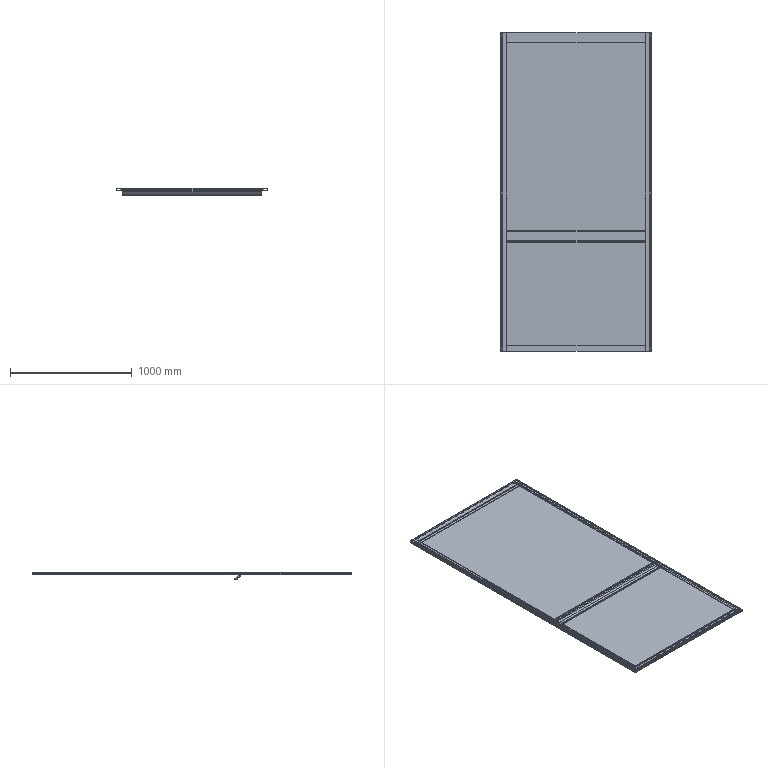Part | 13 solids | 642 faces | box 1240 x 2616 x 63.186 mm | volume 31579551 mm3 | plane 384 | cylinder 258 | commonest cylinder face diameters 1 x56 9 x40 0.4 x34 4 x26 13 x20 14 x20